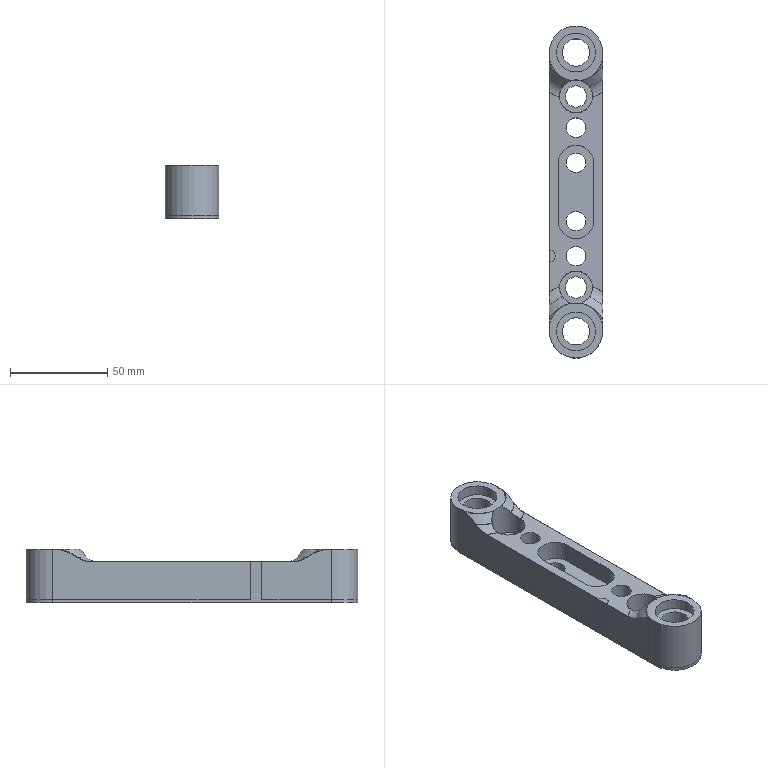Part | 2 solids | 81 faces | box 27.4 x 170.48 x 27.5 mm | volume 146899 mm3 | cylinder 33 | plane 30 | cone 10 | torus 8 | commonest cylinder face diameters 10 x8 11 x4 14 x4 17 x4 18 x4 20 x4